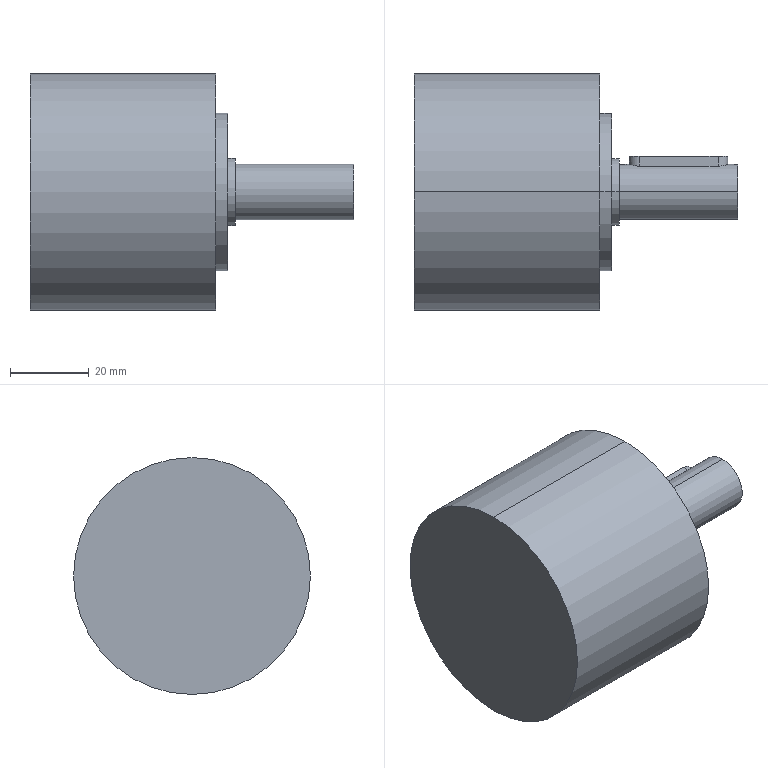Part | STEP file | _PLE60-5_MOTOR(Housing 1-1-3) | 1 solid | 54 faces | box 82 x 60 x 60 mm | volume 141092 mm3 | cone 24 | cylinder 22 | plane 8 | commonest cylinder face diameters 4.134 x8 4.2 x2 5 x2 5.3 x2 14 x2 17 x2